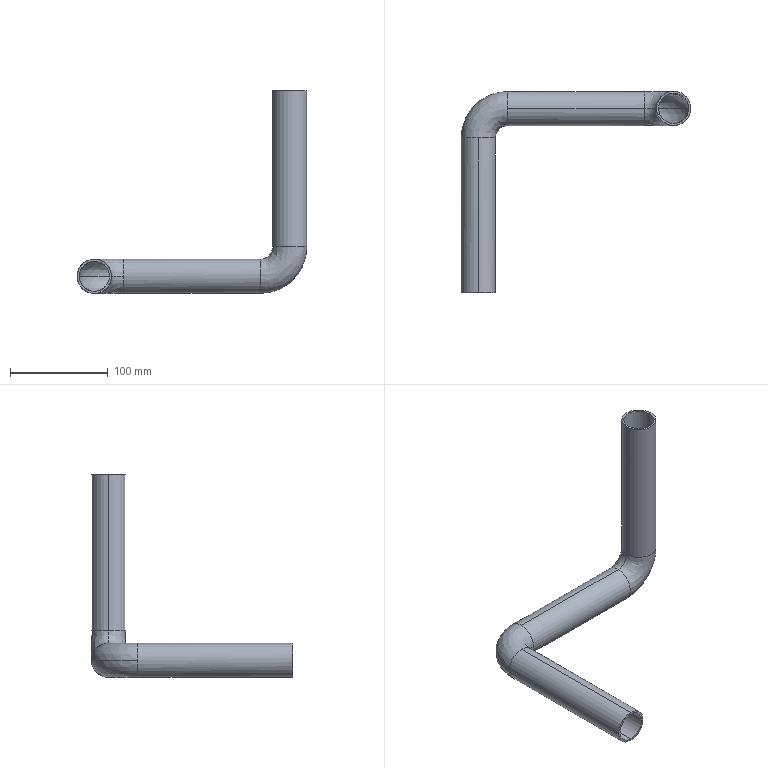Part | STEP file | copper tube 3_default_machined_ | 1 solid | 22 faces | box 235 x 205.85 x 207.5 mm | volume 114578 mm3 | cylinder 12 | spline 8 | plane 2 | commonest cylinder face diameters 31 x6 35 x6